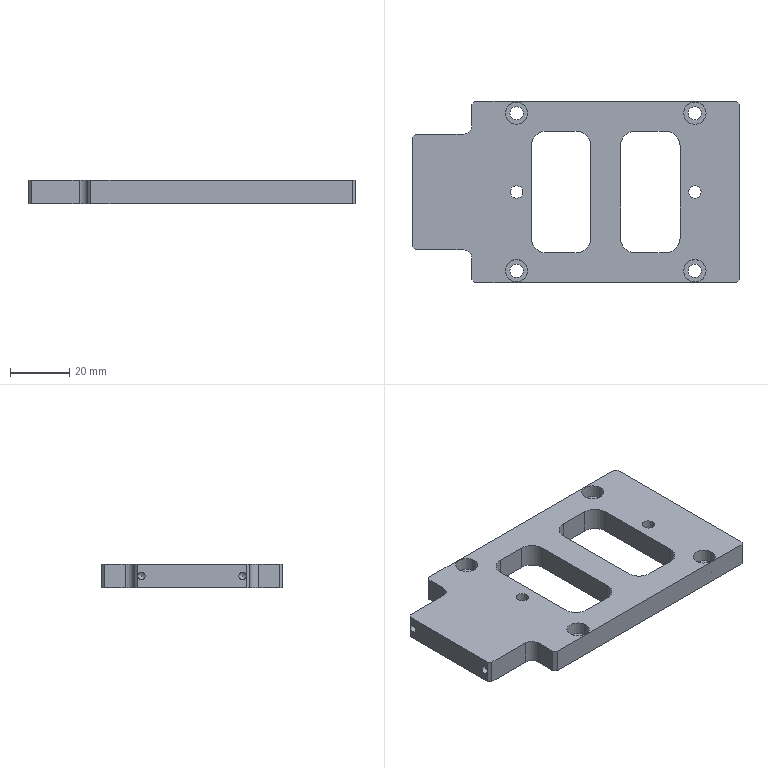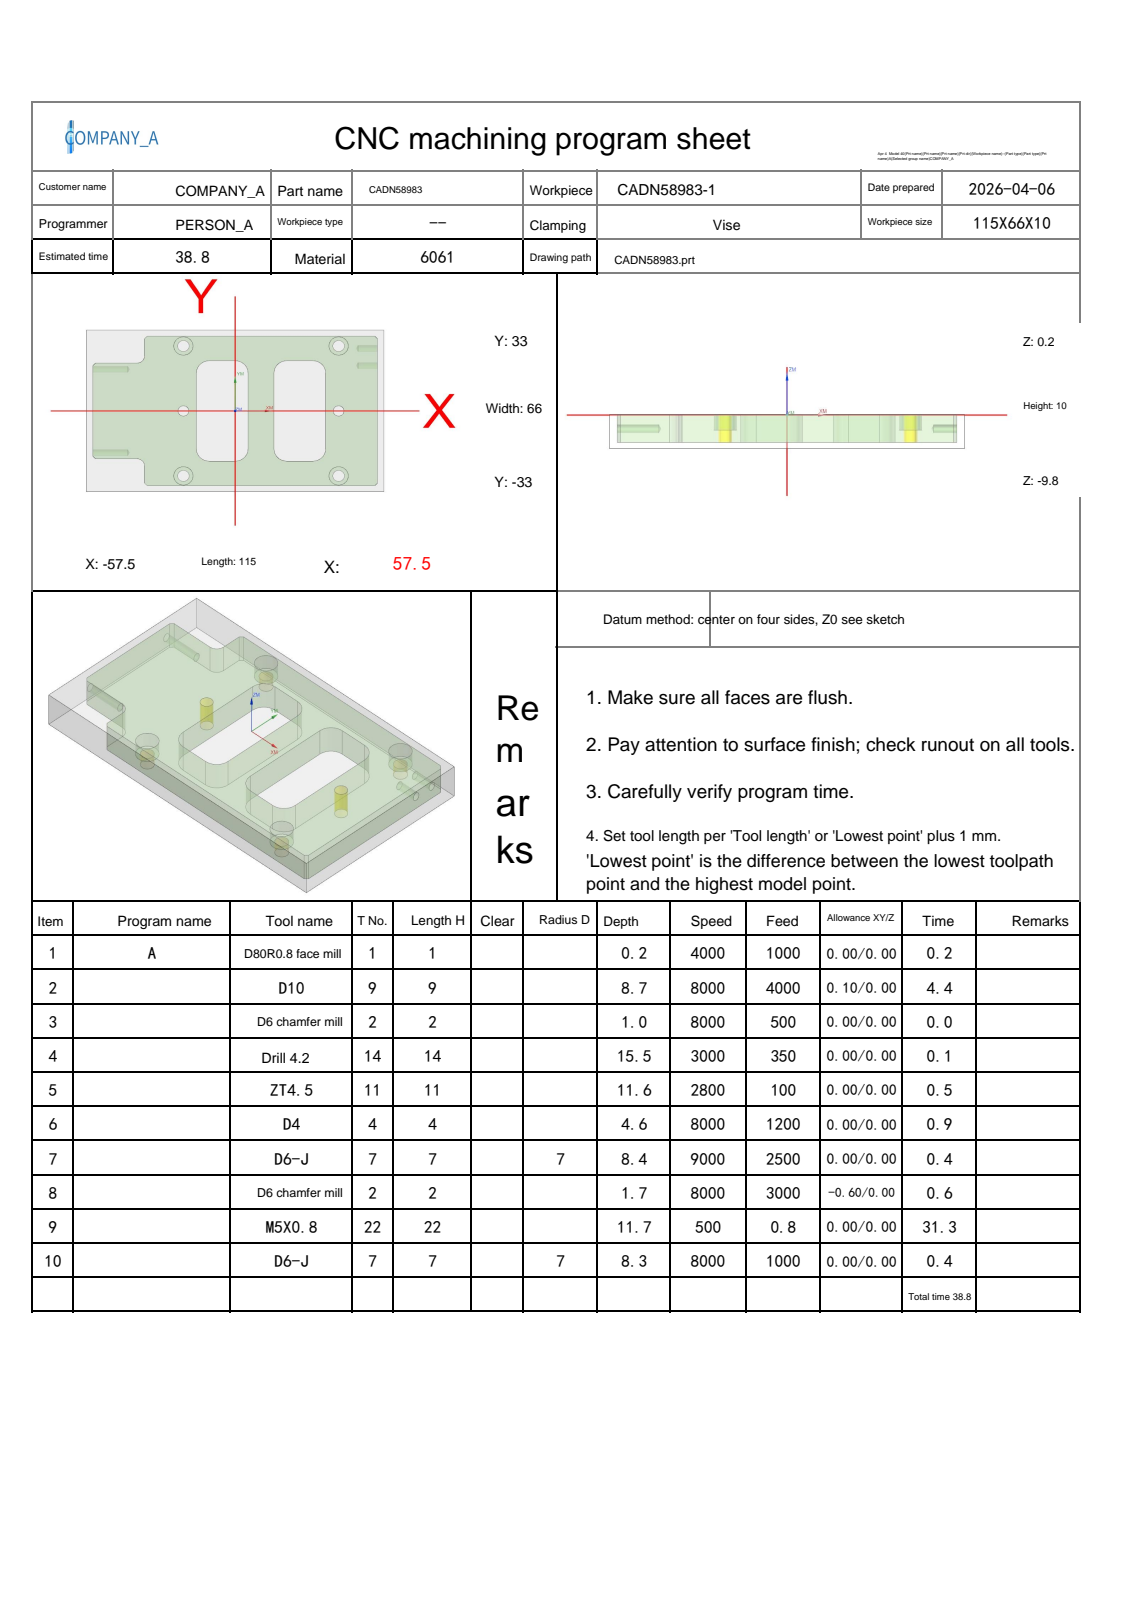NC program | NX | posted by the shop | part box 110 x 61 x 8 mm
Lines 2241 to 4150 of 4510, first 1482 of 1910 lines:
N4 T14 M06
(Drill 4.2 D=4.2 DR_a=118 H=14)
G00 G90 G54 X-20. Y0.0 M03 S3000
G43 H14 Z20.
M08
G98 G83 X-20. Y0.0 Z-15.262 R1. F350. Q3.
X40.
G80
G00 Z20.
G91 G28 Z0.0
M05
M09
G91 G28 Z0.0
M01
N5 T11 M06
(ZT4.5 D=4.5 DR_a=118 H=11)
G00 G90 G54 X40. Y26.5 M03 S2800
G43 H11 Z20.
M08
G98 G83 X40. Y26.5 Z-11.352 R1. F100. Q2.
Y-26.5
X-20.
Y26.5
G80
G00 Z20.
G91 G28 Z0.0
M05
M09
G91 G28 Z0.0
M01
N6 T04 M06
(D4  D=4. R=0. H=04 ce=0.10 di=0.00)
G00 G90 G54 X40. Y26.5 M03 S8000
G43 H04 Z20.
M08
Z.5
G03 X40.825 Y25.675 I.825 J0.0 F1200.
X41.65 Y26.5 I0.0 J.825
X41.65 Y26.5 Z.2 I-1.65 J0.0
X41.65 Y26.5 Z-.1 I-1.65 J0.0
X41.65 Y26.5 Z-.4 I-1.65 J0.0
X41.65 Y26.5 Z-.7 I-1.65 J0.0
X41.65 Y26.5 Z-1. I-1.65 J0.0
X41.65 Y26.5 Z-1.3 I-1.65 J0.0
X41.65 Y26.5 Z-1.6 I-1.65 J0.0
X41.65 Y26.5 Z-1.9 I-1.65 J0.0
X41.65 Y26.5 Z-2.2 I-1.65 J0.0
X41.65 Y26.5 Z-2.5 I-1.65 J0.0
X41.65 Y26.5 Z-2.8 I-1.65 J0.0
X41.65 Y26.5 Z-3.1 I-1.65 J0.0
X41.65 Y26.5 Z-3.4 I-1.65 J0.0
X41.65 Y26.5 Z-3.7 I-1.65 J0.0
X41.65 Y26.5 Z-4. I-1.65 J0.0
X41.65 Y26.5 Z-4.3 I-1.65 J0.0
X39.175 Y27.929 Z-4.4 I-1.65 J0.0
X38.35 Y26.5 I.825 J-1.429
X40. Y24.85 I1.65 J0.0
X41.65 Y26.5 I0.0 J1.65
X40. Y28.15 I-1.65 J0.0
X39.175 Y27.929 I0.0 J-1.65
X38.763 Y27.214 I.413 J-.714
X39.588 Y26.389 I.825 J0.0
X40. Y26.5 I0.0 J.825
G00 Z20.
Y-26.5
Z.5
G03 X40.825 Y-27.325 I.825 J0.0
X41.65 Y-26.5 I0.0 J.825
X41.65 Y-26.5 Z.2 I-1.65 J0.0
X41.65 Y-26.5 Z-.1 I-1.65 J0.0
X41.65 Y-26.5 Z-.4 I-1.65 J0.0
X41.65 Y-26.5 Z-.7 I-1.65 J0.0
X41.65 Y-26.5 Z-1. I-1.65 J0.0
X41.65 Y-26.5 Z-1.3 I-1.65 J0.0
X41.65 Y-26.5 Z-1.6 I-1.65 J0.0
X41.65 Y-26.5 Z-1.9 I-1.65 J0.0
X41.65 Y-26.5 Z-2.2 I-1.65 J0.0
X41.65 Y-26.5 Z-2.5 I-1.65 J0.0
X41.65 Y-26.5 Z-2.8 I-1.65 J0.0
X41.65 Y-26.5 Z-3.1 I-1.65 J0.0
X41.65 Y-26.5 Z-3.4 I-1.65 J0.0
X41.65 Y-26.5 Z-3.7 I-1.65 J0.0
X41.65 Y-26.5 Z-4. I-1.65 J0.0
X41.65 Y-26.5 Z-4.3 I-1.65 J0.0
X39.175 Y-25.071 Z-4.4 I-1.65 J0.0
X38.35 Y-26.5 I.825 J-1.429
X40. Y-28.15 I1.65 J0.0
X41.65 Y-26.5 I0.0 J1.65
X40. Y-24.85 I-1.65 J0.0
X39.175 Y-25.071 I0.0 J-1.65
X38.763 Y-25.786 I.413 J-.714
X39.588 Y-26.611 I.825 J0.0
X40. Y-26.5 I0.0 J.825
G00 Z20.
X-20.
Z.5
G03 X-19.175 Y-27.325 I.825 J0.0
X-18.35 Y-26.5 I0.0 J.825
X-18.35 Y-26.5 Z.2 I-1.65 J0.0
X-18.35 Y-26.5 Z-.1 I-1.65 J0.0
X-18.35 Y-26.5 Z-.4 I-1.65 J0.0
X-18.35 Y-26.5 Z-.7 I-1.65 J0.0
X-18.35 Y-26.5 Z-1. I-1.65 J0.0
X-18.35 Y-26.5 Z-1.3 I-1.65 J0.0
X-18.35 Y-26.5 Z-1.6 I-1.65 J0.0
X-18.35 Y-26.5 Z-1.9 I-1.65 J0.0
X-18.35 Y-26.5 Z-2.2 I-1.65 J0.0
X-18.35 Y-26.5 Z-2.5 I-1.65 J0.0
X-18.35 Y-26.5 Z-2.8 I-1.65 J0.0
X-18.35 Y-26.5 Z-3.1 I-1.65 J0.0
X-18.35 Y-26.5 Z-3.4 I-1.65 J0.0
X-18.35 Y-26.5 Z-3.7 I-1.65 J0.0
X-18.35 Y-26.5 Z-4. I-1.65 J0.0
X-18.35 Y-26.5 Z-4.3 I-1.65 J0.0
X-20.825 Y-25.071 Z-4.4 I-1.65 J0.0
X-21.65 Y-26.5 I.825 J-1.429
X-20. Y-28.15 I1.65 J0.0
X-18.35 Y-26.5 I0.0 J1.65
X-20. Y-24.85 I-1.65 J0.0
X-20.825 Y-25.071 I0.0 J-1.65
X-21.238 Y-25.786 I.413 J-.714
X-20.413 Y-26.611 I.825 J0.0
X-20. Y-26.5 I0.0 J.825
G00 Z20.
Y26.5
Z.5
G03 X-19.175 Y25.675 I.825 J0.0
X-18.35 Y26.5 I0.0 J.825
X-18.35 Y26.5 Z.2 I-1.65 J0.0
X-18.35 Y26.5 Z-.1 I-1.65 J0.0
X-18.35 Y26.5 Z-.4 I-1.65 J0.0
X-18.35 Y26.5 Z-.7 I-1.65 J0.0
X-18.35 Y26.5 Z-1. I-1.65 J0.0
X-18.35 Y26.5 Z-1.3 I-1.65 J0.0
X-18.35 Y26.5 Z-1.6 I-1.65 J0.0
X-18.35 Y26.5 Z-1.9 I-1.65 J0.0
X-18.35 Y26.5 Z-2.2 I-1.65 J0.0
X-18.35 Y26.5 Z-2.5 I-1.65 J0.0
X-18.35 Y26.5 Z-2.8 I-1.65 J0.0
X-18.35 Y26.5 Z-3.1 I-1.65 J0.0
X-18.35 Y26.5 Z-3.4 I-1.65 J0.0
X-18.35 Y26.5 Z-3.7 I-1.65 J0.0
X-18.35 Y26.5 Z-4. I-1.65 J0.0
X-18.35 Y26.5 Z-4.3 I-1.65 J0.0
X-20.825 Y27.929 Z-4.4 I-1.65 J0.0
X-21.65 Y26.5 I.825 J-1.429
X-20. Y24.85 I1.65 J0.0
X-18.35 Y26.5 I0.0 J1.65
X-20. Y28.15 I-1.65 J0.0
X-20.825 Y27.929 I0.0 J-1.65
X-21.238 Y27.214 I.413 J-.714
X-20.413 Y26.389 I.825 J0.0
X-20. Y26.5 I0.0 J.825
G00 Z20.
G00 G90 X40. Y26.5 M03 S8000
Z20.
Z.5
G41 D04
G01 X40.045 Y26.305 F500.
G03 X40.886 Y25.636 I.841 J.195
X41.75 Y26.5 I0.0 J.864
X41.736 Y26.281 Z-4.4 I-1.75 J0.0
X41.75 Y26.5 I-1.736 J.219
X40. Y28.25 I-1.75 J0.0
X38.25 Y26.5 I0.0 J-1.75
X40. Y24.75 I1.75 J0.0
X41.736 Y26.281 I0.0 J1.75
G01 X41.743 Y26.389
G03 X40.879 Y27.252 I-.864 J0.0
X40.069 Y26.688 I0.0 J-.864
G01 G40 X40. Y26.5
G00 Z20.
Y-26.5
Z.5
G41 D04
G01 X40.045 Y-26.695
G03 X40.886 Y-27.364 I.841 J.195
X41.75 Y-26.5 I0.0 J.864
X41.736 Y-26.719 Z-4.4 I-1.75 J0.0
X41.75 Y-26.5 I-1.736 J.219
X40. Y-24.75 I-1.75 J0.0
X38.25 Y-26.5 I0.0 J-1.75
X40. Y-28.25 I1.75 J0.0
X41.736 Y-26.719 I0.0 J1.75
G01 X41.743 Y-26.611
G03 X40.879 Y-25.748 I-.864 J0.0
X40.069 Y-26.312 I0.0 J-.864
G01 G40 X40. Y-26.5
G00 Z20.
X-20.
Z.5
G41 D04
G01 X-19.955 Y-26.695
G03 X-19.114 Y-27.364 I.841 J.195
X-18.25 Y-26.5 I0.0 J.864
X-18.264 Y-26.719 Z-4.4 I-1.75 J0.0
X-18.25 Y-26.5 I-1.736 J.219
X-20. Y-24.75 I-1.75 J0.0
X-21.75 Y-26.5 I0.0 J-1.75
X-20. Y-28.25 I1.75 J0.0
X-18.264 Y-26.719 I0.0 J1.75
G01 X-18.257 Y-26.611
G03 X-19.121 Y-25.748 I-.864 J0.0
X-19.931 Y-26.312 I0.0 J-.864
G01 G40 X-20. Y-26.5
G00 Z20.
Y26.5
Z.5
G41 D04
G01 X-19.955 Y26.305
G03 X-19.114 Y25.636 I.841 J.195
X-18.25 Y26.5 I0.0 J.864
X-18.264 Y26.281 Z-4.4 I-1.75 J0.0
X-18.25 Y26.5 I-1.736 J.219
X-20. Y28.25 I-1.75 J0.0
X-21.75 Y26.5 I0.0 J-1.75
X-20. Y24.75 I1.75 J0.0
X-18.264 Y26.281 I0.0 J1.75
G01 X-18.257 Y26.389
G03 X-19.121 Y27.252 I-.864 J0.0
X-19.931 Y26.688 I0.0 J-.864
G01 G40 X-20. Y26.5
G00 Z20.
G91 G28 Z0.0
M05
M09
G91 G28 Z0.0
M01
N7 T07 M06
(D6-J  D=6. R=0. H=07 ce=0.00 di=0.00)
G00 G90 G54 X29.9 Y-16.5 M03 S6000
G43 H07 Z20.
M08
Z-7.7
G01 Z-8.2 F1000.
G41 D07
X31.
G03 X32. Y-15.5 I0.0 J1.
G01 Y15.5
G03 X30. Y17.5 I-2. J0.0
G01 X20.
G03 X18. Y15.5 I0.0 J-2.
G01 Y-15.5
G03 X20. Y-17.5 I2. J0.0
G01 X30.
G03 X32. Y-15.5 I0.0 J2.
G01 Y-15.
G03 X31. Y-14. I-1. J0.0
G01 G40 X30.9
Z-7.7
G00 Z20.
X-.1 Y-16.5
Z-7.7
G01 Z-8.2
G41 D07
X1.
G03 X2. Y-15.5 I0.0 J1.
G01 Y15.5
G03 X0.0 Y17.5 I-2. J0.0
G01 X-10.
G03 X-12. Y15.5 I0.0 J-2.
G01 Y-15.5
G03 X-10. Y-17.5 I2. J0.0
G01 X0.0
G03 X2. Y-15.5 I0.0 J2.
G01 Y-15.
G03 X1. Y-14. I-1. J0.0
G01 G40 X.9
Z-7.7
G00 Z20.
G00 G90 X-38.919 Y-25.318 M03 S9000
Z20.
Z.606
G01 X-38.909 Y-25.316 Z.477 F2000.
X-38.88 Y-25.312 Z.36
X-38.834 Y-25.303 Z.255
X-38.776 Y-25.291 Z.161
X-38.706 Y-25.275 Z.078
X-38.628 Y-25.254 Z.004
X-38.545 Y-25.228 Z-.06
X-38.46 Y-25.197 Z-.114
X-38.374 Y-25.16 Z-.161
X-38.291 Y-25.118 Z-.2
X-38.213 Y-25.069 Z-.231
X-38.144 Y-25.013 Z-.255
X-38.085 Y-24.95 Z-.273
X-38.039 Y-24.88 Z-.285
X-38.01 Y-24.802 Z-.292
X-38. Y-24.716 Z-.294
Y-22.5 F2500.
X-40.216
X-40.289 Y-22.516 Z-.295
X-40.343 Y-22.563 Z-.298
X-40.381 Y-22.636 Z-.302
X-40.403 Y-22.732 Z-.308
X-40.411 Y-22.845 Z-.314
X-40.406 Y-22.974 Z-.322
X-40.389 Y-23.112 Z-.331
X-40.362 Y-23.258 Z-.341
X-40.325 Y-23.406 Z-.352
X-40.28 Y-23.553 Z-.363
X-40.228 Y-23.694 Z-.374
X-40.117 Y-23.932 Z-.396
X-39.985 Y-24.14 Z-.419
X-39.83 Y-24.321 Z-.442
X-39.649 Y-24.478 Z-.465
X-39.441 Y-24.611 Z-.487
X-39.203 Y-24.723 Z-.509
X-39.061 Y-24.776 Z-.521
X-38.913 Y-24.821 Z-.532
X-38.764 Y-24.859 Z-.542
X-38.618 Y-24.887 Z-.552
X-38.478 Y-24.905 Z-.561
X-38.349 Y-24.91 Z-.569
X-38.234 Y-24.903 Z-.576
X-38.137 Y-24.881 Z-.581
X-38.064 Y-24.843 Z-.585
X-38.017 Y-24.789 Z-.588
X-38. Y-24.716 Z-.589
Y-22.5
X-40.216
X-40.289 Y-22.516 Z-.59
X-40.343 Y-22.563 Z-.592
X-40.381 Y-22.636 Z-.596
X-40.403 Y-22.732 Z-.602
X-40.411 Y-22.845 Z-.609
X-40.406 Y-22.974 Z-.617
X-40.389 Y-23.112 Z-.626
X-40.362 Y-23.258 Z-.635
X-40.325 Y-23.406 Z-.646
X-40.28 Y-23.553 Z-.657
X-40.228 Y-23.694 Z-.669
X-40.117 Y-23.932 Z-.691
X-39.985 Y-24.14 Z-.713
X-39.83 Y-24.321 Z-.736
X-39.649 Y-24.478 Z-.759
X-39.441 Y-24.611 Z-.782
X-39.203 Y-24.723 Z-.804
X-39.061 Y-24.776 Z-.815
X-38.913 Y-24.821 Z-.826
X-38.764 Y-24.859 Z-.837
X-38.618 Y-24.887 Z-.847
X-38.478 Y-24.905 Z-.855
X-38.349 Y-24.91 Z-.863
X-38.234 Y-24.903 Z-.87
X-38.137 Y-24.881 Z-.876
X-38.064 Y-24.843 Z-.88
X-38.017 Y-24.789 Z-.882
X-38. Y-24.716 Z-.883
Y-22.5
X-40.216
X-40.289 Y-22.516 Z-.884
X-40.343 Y-22.563 Z-.887
X-40.381 Y-22.636 Z-.891
X-40.403 Y-22.732 Z-.896
X-40.411 Y-22.845 Z-.903
X-40.406 Y-22.974 Z-.911
X-40.389 Y-23.112 Z-.92
X-40.362 Y-23.258 Z-.93
X-40.325 Y-23.406 Z-.94
X-40.28 Y-23.553 Z-.952
X-40.228 Y-23.694 Z-.963
X-40.117 Y-23.932 Z-.985
X-39.985 Y-24.14 Z-1.008
X-39.83 Y-24.321 Z-1.031
X-39.649 Y-24.478 Z-1.054
X-39.441 Y-24.611 Z-1.076
X-39.203 Y-24.723 Z-1.098
X-39.061 Y-24.776 Z-1.11
X-38.913 Y-24.821 Z-1.121
X-38.764 Y-24.859 Z-1.131
X-38.618 Y-24.887 Z-1.141
X-38.478 Y-24.905 Z-1.15
X-38.349 Y-24.91 Z-1.158
X-38.234 Y-24.903 Z-1.165
X-38.137 Y-24.881 Z-1.17
X-38.064 Y-24.843 Z-1.174
X-38.017 Y-24.789 Z-1.177
X-38. Y-24.716 Z-1.178
Y-22.5
X-40.216
X-40.289 Y-22.516 Z-1.179
X-40.343 Y-22.563 Z-1.181
X-40.381 Y-22.636 Z-1.185
X-40.403 Y-22.732 Z-1.191
X-40.411 Y-22.845 Z-1.198
X-40.406 Y-22.974 Z-1.206
X-40.389 Y-23.112 Z-1.215
X-40.362 Y-23.258 Z-1.224
X-40.325 Y-23.406 Z-1.235
X-40.28 Y-23.553 Z-1.246
X-40.228 Y-23.694 Z-1.258
X-40.117 Y-23.932 Z-1.279
X-39.985 Y-24.14 Z-1.302
X-39.83 Y-24.321 Z-1.325
X-39.649 Y-24.478 Z-1.348
X-39.441 Y-24.611 Z-1.371
X-39.203 Y-24.723 Z-1.392
X-39.061 Y-24.776 Z-1.404
X-38.913 Y-24.821 Z-1.415
X-38.764 Y-24.859 Z-1.426
X-38.618 Y-24.887 Z-1.435
X-38.478 Y-24.905 Z-1.444
X-38.349 Y-24.91 Z-1.452
X-38.234 Y-24.903 Z-1.459
X-38.137 Y-24.881 Z-1.465
X-38.064 Y-24.843 Z-1.469
X-38.017 Y-24.789 Z-1.471
X-38. Y-24.716 Z-1.472
Y-22.5
X-40.216
X-40.289 Y-22.516 Z-1.473
X-40.343 Y-22.563 Z-1.476
X-40.381 Y-22.636 Z-1.48
X-40.403 Y-22.732 Z-1.485
X-40.411 Y-22.845 Z-1.492
X-40.406 Y-22.974 Z-1.5
X-40.389 Y-23.112 Z-1.509
X-40.362 Y-23.258 Z-1.519
X-40.325 Y-23.406 Z-1.529
X-40.28 Y-23.553 Z-1.54
X-40.228 Y-23.694 Z-1.552
X-40.117 Y-23.932 Z-1.574
X-39.985 Y-24.14 Z-1.596
X-39.83 Y-24.321 Z-1.619
X-39.649 Y-24.478 Z-1.642
X-39.441 Y-24.611 Z-1.665
X-39.203 Y-24.723 Z-1.687
X-39.061 Y-24.776 Z-1.698
X-38.913 Y-24.821 Z-1.71
X-38.764 Y-24.859 Z-1.72
X-38.618 Y-24.887 Z-1.73
X-38.478 Y-24.905 Z-1.739
X-38.349 Y-24.91 Z-1.747
X-38.234 Y-24.903 Z-1.754
X-38.137 Y-24.881 Z-1.759
X-38.064 Y-24.843 Z-1.763
X-38.017 Y-24.789 Z-1.766
X-38. Y-24.716 Z-1.767
Y-22.5
X-40.216
X-40.289 Y-22.516 Z-1.768
X-40.343 Y-22.563 Z-1.77
X-40.381 Y-22.636 Z-1.774
X-40.403 Y-22.732 Z-1.78
X-40.411 Y-22.845 Z-1.787
X-40.406 Y-22.974 Z-1.795
X-40.389 Y-23.112 Z-1.803
X-40.362 Y-23.258 Z-1.813
X-40.325 Y-23.406 Z-1.824
X-40.28 Y-23.553 Z-1.835
X-40.228 Y-23.694 Z-1.846
X-40.117 Y-23.932 Z-1.868
X-39.985 Y-24.14 Z-1.891
X-39.83 Y-24.321 Z-1.914
X-39.649 Y-24.478 Z-1.937
X-39.441 Y-24.611 Z-1.959
X-39.203 Y-24.723 Z-1.981
X-39.061 Y-24.776 Z-1.993
X-38.913 Y-24.821 Z-2.004
X-38.764 Y-24.859 Z-2.015
X-38.618 Y-24.887 Z-2.024
X-38.478 Y-24.905 Z-2.033
X-38.349 Y-24.91 Z-2.041
X-38.234 Y-24.903 Z-2.048
X-38.137 Y-24.881 Z-2.054
X-38.064 Y-24.843 Z-2.058
X-38.017 Y-24.789 Z-2.06
X-38. Y-24.716 Z-2.061
Y-22.5
X-40.216
X-40.289 Y-22.516 Z-2.062
X-40.343 Y-22.563 Z-2.065
X-40.381 Y-22.636 Z-2.069
X-40.403 Y-22.732 Z-2.074
X-40.411 Y-22.845 Z-2.081
X-40.406 Y-22.974 Z-2.089
X-40.389 Y-23.112 Z-2.098
X-40.362 Y-23.258 Z-2.108
X-40.325 Y-23.406 Z-2.118
X-40.28 Y-23.553 Z-2.129
X-40.228 Y-23.694 Z-2.141
X-40.117 Y-23.932 Z-2.163
X-39.985 Y-24.14 Z-2.185
X-39.83 Y-24.321 Z-2.208
X-39.649 Y-24.478 Z-2.231
X-39.441 Y-24.611 Z-2.254
X-39.203 Y-24.723 Z-2.276
X-39.061 Y-24.776 Z-2.287
X-38.913 Y-24.821 Z-2.298
X-38.764 Y-24.859 Z-2.309
X-38.618 Y-24.887 Z-2.319
X-38.478 Y-24.905 Z-2.328
X-38.349 Y-24.91 Z-2.336
X-38.234 Y-24.903 Z-2.342
X-38.137 Y-24.881 Z-2.348
X-38.064 Y-24.843 Z-2.352
X-38.017 Y-24.789 Z-2.355
X-38. Y-24.716 Z-2.356
Y-22.5
X-40.216
X-40.289 Y-22.516
X-40.343 Y-22.563 Z-2.359
X-40.381 Y-22.636 Z-2.363
X-40.403 Y-22.732 Z-2.369
X-40.411 Y-22.845 Z-2.375
X-40.406 Y-22.974 Z-2.383
X-40.389 Y-23.112 Z-2.392
X-40.362 Y-23.258 Z-2.402
X-40.325 Y-23.406 Z-2.413
X-40.28 Y-23.553 Z-2.424
X-40.228 Y-23.694 Z-2.435
X-40.117 Y-23.932 Z-2.457
X-39.985 Y-24.14 Z-2.48
X-39.83 Y-24.321 Z-2.503
X-39.649 Y-24.478 Z-2.526
X-39.441 Y-24.611 Z-2.548
X-39.203 Y-24.723 Z-2.57
X-39.061 Y-24.776 Z-2.582
X-38.913 Y-24.821 Z-2.593
X-38.764 Y-24.859 Z-2.603
X-38.618 Y-24.887 Z-2.613
X-38.478 Y-24.905 Z-2.622
X-38.349 Y-24.91 Z-2.63
X-38.234 Y-24.903 Z-2.637
X-38.137 Y-24.881 Z-2.642
X-38.064 Y-24.843 Z-2.647
X-38.017 Y-24.789 Z-2.649
X-38. Y-24.716 Z-2.65
Y-22.5
X-40.216
X-40.289 Y-22.516 Z-2.651
X-40.343 Y-22.563 Z-2.653
X-40.381 Y-22.636 Z-2.658
X-40.403 Y-22.732 Z-2.663
X-40.411 Y-22.845 Z-2.67
X-40.406 Y-22.974 Z-2.678
X-40.389 Y-23.112 Z-2.687
X-40.362 Y-23.258 Z-2.697
X-40.325 Y-23.406 Z-2.707
X-40.28 Y-23.553 Z-2.718
X-40.228 Y-23.694 Z-2.73
X-40.117 Y-23.932 Z-2.752
X-39.985 Y-24.14 Z-2.774
X-39.83 Y-24.321 Z-2.797
X-39.649 Y-24.478 Z-2.82
X-39.441 Y-24.611 Z-2.843
X-39.203 Y-24.723 Z-2.865
X-39.061 Y-24.776 Z-2.876
X-38.913 Y-24.821 Z-2.887
X-38.764 Y-24.859 Z-2.898
X-38.618 Y-24.887 Z-2.908
X-38.478 Y-24.905 Z-2.917
X-38.349 Y-24.91 Z-2.925
X-38.234 Y-24.903 Z-2.931
X-38.137 Y-24.881 Z-2.937
X-38.064 Y-24.843 Z-2.941
X-38.017 Y-24.789 Z-2.944
X-38. Y-24.716
Y-22.5
X-40.216
X-40.289 Y-22.516 Z-2.945
X-40.343 Y-22.563 Z-2.948
X-40.381 Y-22.636 Z-2.952
X-40.403 Y-22.732 Z-2.958
X-40.411 Y-22.845 Z-2.964
X-40.406 Y-22.974 Z-2.972
X-40.389 Y-23.112 Z-2.981
X-40.362 Y-23.258 Z-2.991
X-40.325 Y-23.406 Z-3.002
X-40.28 Y-23.553 Z-3.013
X-40.228 Y-23.694 Z-3.024
X-40.117 Y-23.932 Z-3.046
X-39.985 Y-24.14 Z-3.069
X-39.83 Y-24.321 Z-3.092
X-39.649 Y-24.478 Z-3.115
X-39.441 Y-24.611 Z-3.137
X-39.203 Y-24.723 Z-3.159
X-39.061 Y-24.776 Z-3.171
X-38.913 Y-24.821 Z-3.182
X-38.764 Y-24.859 Z-3.192
X-38.618 Y-24.887 Z-3.202
X-38.478 Y-24.905 Z-3.211
X-38.349 Y-24.91 Z-3.219
X-38.234 Y-24.903 Z-3.226
X-38.137 Y-24.881 Z-3.231
X-38.064 Y-24.843 Z-3.235
X-38.017 Y-24.789 Z-3.238
X-38. Y-24.716 Z-3.239
Y-22.5
X-40.216
X-40.289 Y-22.516 Z-3.24
X-40.343 Y-22.563 Z-3.242
X-40.381 Y-22.636 Z-3.246
X-40.403 Y-22.732 Z-3.252
X-40.411 Y-22.845 Z-3.259
X-40.406 Y-22.974 Z-3.267
X-40.389 Y-23.112 Z-3.276
X-40.362 Y-23.258 Z-3.285
X-40.325 Y-23.406 Z-3.296
X-40.28 Y-23.553 Z-3.307
X-40.228 Y-23.694 Z-3.319
X-40.117 Y-23.932 Z-3.341
X-39.985 Y-24.14 Z-3.363
X-39.83 Y-24.321 Z-3.386
X-39.649 Y-24.478 Z-3.409
X-39.441 Y-24.611 Z-3.432
X-39.203 Y-24.723 Z-3.454
X-39.061 Y-24.776 Z-3.465
X-38.913 Y-24.821 Z-3.476
X-38.764 Y-24.859 Z-3.487
X-38.618 Y-24.887 Z-3.497
X-38.478 Y-24.905 Z-3.505
X-38.349 Y-24.91 Z-3.513
X-38.234 Y-24.903 Z-3.52
X-38.137 Y-24.881 Z-3.526
X-38.064 Y-24.843 Z-3.53
X-38.017 Y-24.789 Z-3.532
X-38. Y-24.716 Z-3.533
Y-22.5
X-40.216
X-40.289 Y-22.516 Z-3.534
X-40.343 Y-22.563 Z-3.537
X-40.381 Y-22.636 Z-3.541
X-40.403 Y-22.732 Z-3.546
X-40.411 Y-22.845 Z-3.553
X-40.406 Y-22.974 Z-3.561
X-40.389 Y-23.112 Z-3.57
X-40.362 Y-23.258 Z-3.58
X-40.325 Y-23.406 Z-3.59
X-40.28 Y-23.553 Z-3.602
X-40.228 Y-23.694 Z-3.613
X-40.117 Y-23.932 Z-3.635
X-39.985 Y-24.14 Z-3.658
X-39.83 Y-24.321 Z-3.681
X-39.649 Y-24.478 Z-3.704
X-39.441 Y-24.611 Z-3.726
X-39.203 Y-24.723 Z-3.748
X-39.061 Y-24.776 Z-3.76
X-38.913 Y-24.821 Z-3.771
X-38.764 Y-24.859 Z-3.781
X-38.618 Y-24.887 Z-3.791
X-38.478 Y-24.905 Z-3.8
X-38.349 Y-24.91 Z-3.808
X-38.234 Y-24.903 Z-3.815
X-38.137 Y-24.881 Z-3.82
X-38.064 Y-24.843 Z-3.824
X-38.017 Y-24.789 Z-3.827
X-38. Y-24.716 Z-3.828
Y-22.5
X-40.216
X-40.289 Y-22.516 Z-3.829
X-40.343 Y-22.563 Z-3.831
X-40.381 Y-22.636 Z-3.835
X-40.403 Y-22.732 Z-3.841
X-40.411 Y-22.845 Z-3.848
X-40.406 Y-22.974 Z-3.856
X-40.389 Y-23.112 Z-3.865
X-40.362 Y-23.258 Z-3.874
X-40.325 Y-23.406 Z-3.885
X-40.28 Y-23.553 Z-3.896
X-40.228 Y-23.694 Z-3.908
X-40.117 Y-23.932 Z-3.929
X-39.985 Y-24.14 Z-3.952
X-39.83 Y-24.321 Z-3.975
X-39.649 Y-24.478 Z-3.998
X-39.441 Y-24.611 Z-4.021
X-39.203 Y-24.723 Z-4.042
X-39.061 Y-24.776 Z-4.054
X-38.913 Y-24.821 Z-4.065
X-38.764 Y-24.859 Z-4.076
X-38.618 Y-24.887 Z-4.085
X-38.478 Y-24.905 Z-4.094
X-38.349 Y-24.91 Z-4.102
X-38.234 Y-24.903 Z-4.109
X-38.137 Y-24.881 Z-4.115
X-38.064 Y-24.843 Z-4.119
X-38.017 Y-24.789 Z-4.121
X-38. Y-24.716 Z-4.122
Y-22.5
X-40.216
X-40.289 Y-22.516 Z-4.123
X-40.343 Y-22.563 Z-4.126
X-40.381 Y-22.636 Z-4.13
X-40.403 Y-22.732 Z-4.135
X-40.411 Y-22.845 Z-4.142
X-40.406 Y-22.974 Z-4.15
X-40.389 Y-23.112 Z-4.159
X-40.362 Y-23.258 Z-4.169
X-40.325 Y-23.406 Z-4.179
X-40.28 Y-23.553 Z-4.19
X-40.228 Y-23.694 Z-4.202
X-40.117 Y-23.932 Z-4.224
X-39.985 Y-24.14 Z-4.246
X-39.83 Y-24.321 Z-4.269
X-39.649 Y-24.478 Z-4.292
X-39.441 Y-24.611 Z-4.315
X-39.203 Y-24.723 Z-4.337
X-39.061 Y-24.776 Z-4.348
X-38.913 Y-24.821 Z-4.36
X-38.764 Y-24.859 Z-4.37
X-38.618 Y-24.887 Z-4.38
X-38.478 Y-24.905 Z-4.389
X-38.349 Y-24.91 Z-4.397
X-38.234 Y-24.903 Z-4.404
X-38.137 Y-24.881 Z-4.409
X-38.064 Y-24.843 Z-4.413
X-38.017 Y-24.789 Z-4.416
X-38. Y-24.716 Z-4.417
Y-22.5
X-40.216
X-40.289 Y-22.516 Z-4.418
X-40.343 Y-22.563 Z-4.42
X-40.381 Y-22.636 Z-4.424
X-40.403 Y-22.732 Z-4.43
X-40.411 Y-22.845 Z-4.437
X-40.406 Y-22.974 Z-4.445
X-40.389 Y-23.112 Z-4.453
X-40.362 Y-23.258 Z-4.463
X-40.325 Y-23.406 Z-4.474
X-40.28 Y-23.553 Z-4.485
X-40.228 Y-23.694 Z-4.496
X-40.117 Y-23.932 Z-4.518
X-39.985 Y-24.14 Z-4.541
X-39.83 Y-24.321 Z-4.564
X-39.649 Y-24.478 Z-4.587
X-39.441 Y-24.611 Z-4.609
X-39.203 Y-24.723 Z-4.631
X-39.061 Y-24.776 Z-4.643
X-38.913 Y-24.821 Z-4.654
X-38.764 Y-24.859 Z-4.665
X-38.618 Y-24.887 Z-4.674
X-38.478 Y-24.905 Z-4.683
X-38.349 Y-24.91 Z-4.691
X-38.234 Y-24.903 Z-4.698
X-38.137 Y-24.881 Z-4.704
X-38.064 Y-24.843 Z-4.708
X-38.017 Y-24.789 Z-4.71
X-38. Y-24.716 Z-4.711
Y-22.5
X-40.216
X-40.289 Y-22.516 Z-4.712
X-40.343 Y-22.563 Z-4.715
X-40.381 Y-22.636 Z-4.719
X-40.403 Y-22.732 Z-4.724
X-40.411 Y-22.845 Z-4.731
X-40.406 Y-22.974 Z-4.739
X-40.389 Y-23.112 Z-4.748
X-40.362 Y-23.258 Z-4.758
X-40.325 Y-23.406 Z-4.768
X-40.28 Y-23.553 Z-4.779
X-40.228 Y-23.694 Z-4.791
X-40.117 Y-23.932 Z-4.813
X-39.985 Y-24.14 Z-4.835
X-39.83 Y-24.321 Z-4.858
X-39.649 Y-24.478 Z-4.881
X-39.441 Y-24.611 Z-4.904
X-39.203 Y-24.723 Z-4.926
X-39.061 Y-24.776 Z-4.937
X-38.913 Y-24.821 Z-4.948
X-38.764 Y-24.859 Z-4.959
X-38.618 Y-24.887 Z-4.969
X-38.478 Y-24.905 Z-4.978
X-38.349 Y-24.91 Z-4.986
X-38.234 Y-24.903 Z-4.992
X-38.137 Y-24.881 Z-4.998
X-38.064 Y-24.843 Z-5.002
X-38.017 Y-24.789 Z-5.005
X-38. Y-24.716 Z-5.006
Y-22.5
X-40.216
X-40.289 Y-22.516
X-40.343 Y-22.563 Z-5.009
X-40.381 Y-22.636 Z-5.013
X-40.403 Y-22.732 Z-5.019
X-40.411 Y-22.845 Z-5.025
X-40.406 Y-22.974 Z-5.033
X-40.389 Y-23.112 Z-5.042
X-40.362 Y-23.258 Z-5.052
X-40.325 Y-23.406 Z-5.063
X-40.28 Y-23.553 Z-5.074
X-40.228 Y-23.694 Z-5.085
X-40.117 Y-23.932 Z-5.107
X-39.985 Y-24.14 Z-5.13
X-39.83 Y-24.321 Z-5.153
X-39.649 Y-24.478 Z-5.176
X-39.441 Y-24.611 Z-5.198
X-39.203 Y-24.723 Z-5.22
X-39.061 Y-24.776 Z-5.232
X-38.913 Y-24.821 Z-5.243
X-38.764 Y-24.859 Z-5.253
X-38.618 Y-24.887 Z-5.263
X-38.478 Y-24.905 Z-5.272
X-38.349 Y-24.91 Z-5.28
X-38.234 Y-24.903 Z-5.287
X-38.137 Y-24.881 Z-5.292
X-38.064 Y-24.843 Z-5.297
X-38.017 Y-24.789 Z-5.299
X-38. Y-24.716 Z-5.3
Y-22.5
X-40.216
X-40.289 Y-22.516 Z-5.301
X-40.343 Y-22.563 Z-5.303
X-40.381 Y-22.636 Z-5.308
X-40.403 Y-22.732 Z-5.313
X-40.411 Y-22.845 Z-5.32
X-40.406 Y-22.974 Z-5.328
X-40.389 Y-23.112 Z-5.337
X-40.362 Y-23.258 Z-5.347
X-40.325 Y-23.406 Z-5.357
X-40.28 Y-23.553 Z-5.368
X-40.228 Y-23.694 Z-5.38
X-40.117 Y-23.932 Z-5.402
X-39.985 Y-24.14 Z-5.424
X-39.83 Y-24.321 Z-5.447
X-39.649 Y-24.478 Z-5.47
X-39.441 Y-24.611 Z-5.493
X-39.203 Y-24.723 Z-5.515
X-39.061 Y-24.776 Z-5.526
X-38.913 Y-24.821 Z-5.537
X-38.764 Y-24.859 Z-5.548
X-38.618 Y-24.887 Z-5.558
X-38.478 Y-24.905 Z-5.567
X-38.349 Y-24.91 Z-5.575
X-38.234 Y-24.903 Z-5.581
X-38.137 Y-24.881 Z-5.587
X-38.064 Y-24.843 Z-5.591
X-38.017 Y-24.789 Z-5.594
X-38. Y-24.716
Y-22.5
X-40.216
X-40.289 Y-22.516 Z-5.595
X-40.343 Y-22.563 Z-5.598
X-40.381 Y-22.636 Z-5.602
X-40.403 Y-22.732 Z-5.608
X-40.411 Y-22.845 Z-5.614
X-40.406 Y-22.974 Z-5.622
X-40.389 Y-23.112 Z-5.631
X-40.362 Y-23.258 Z-5.641
X-40.325 Y-23.406 Z-5.652
X-40.28 Y-23.553 Z-5.663
X-40.228 Y-23.694 Z-5.674
X-40.117 Y-23.932 Z-5.696
X-39.985 Y-24.14 Z-5.719
X-39.83 Y-24.321 Z-5.742
X-39.649 Y-24.478 Z-5.765
X-39.441 Y-24.611 Z-5.787
X-39.203 Y-24.723 Z-5.809
X-39.061 Y-24.776 Z-5.821
X-38.913 Y-24.821 Z-5.832
X-38.764 Y-24.859 Z-5.842
X-38.618 Y-24.887 Z-5.852
X-38.478 Y-24.905 Z-5.861
X-38.349 Y-24.91 Z-5.869
X-38.234 Y-24.903 Z-5.876
X-38.137 Y-24.881 Z-5.881
X-38.064 Y-24.843 Z-5.885
X-38.017 Y-24.789 Z-5.888
X-38. Y-24.716 Z-5.889
Y-22.5
X-40.216
X-40.289 Y-22.516 Z-5.89
X-40.343 Y-22.563 Z-5.892
X-40.381 Y-22.636 Z-5.896
X-40.403 Y-22.732 Z-5.902
X-40.411 Y-22.845 Z-5.909
X-40.406 Y-22.974 Z-5.917
X-40.389 Y-23.112 Z-5.926
X-40.362 Y-23.258 Z-5.935
X-40.325 Y-23.406 Z-5.946
X-40.28 Y-23.553 Z-5.957
X-40.228 Y-23.694 Z-5.969
X-40.117 Y-23.932 Z-5.991
X-39.985 Y-24.14 Z-6.013
X-39.83 Y-24.321 Z-6.036
X-39.649 Y-24.478 Z-6.059
X-39.441 Y-24.611 Z-6.082
X-39.203 Y-24.723 Z-6.104
X-39.061 Y-24.776 Z-6.115
X-38.913 Y-24.821 Z-6.126
X-38.764 Y-24.859 Z-6.137
X-38.618 Y-24.887 Z-6.147
X-38.478 Y-24.905 Z-6.155
X-38.349 Y-24.91 Z-6.163
X-38.234 Y-24.903 Z-6.17
X-38.137 Y-24.881 Z-6.176
X-38.064 Y-24.843 Z-6.18
X-38.017 Y-24.789 Z-6.182
X-38. Y-24.716 Z-6.183
Y-22.5
X-40.216
X-40.289 Y-22.516 Z-6.184
X-40.343 Y-22.563 Z-6.187
X-40.381 Y-22.636 Z-6.191
X-40.403 Y-22.732 Z-6.196
X-40.411 Y-22.845 Z-6.203
X-40.406 Y-22.974 Z-6.211
X-40.389 Y-23.112 Z-6.22
X-40.362 Y-23.258 Z-6.23
X-40.325 Y-23.406 Z-6.24
X-40.28 Y-23.553 Z-6.252
X-40.228 Y-23.694 Z-6.263
X-40.117 Y-23.932 Z-6.285
X-39.985 Y-24.14 Z-6.308
X-39.83 Y-24.321 Z-6.331
X-39.649 Y-24.478 Z-6.354
X-39.441 Y-24.611 Z-6.376
X-39.203 Y-24.723 Z-6.398
X-39.061 Y-24.776 Z-6.41
X-38.913 Y-24.821 Z-6.421
X-38.764 Y-24.859 Z-6.431
X-38.618 Y-24.887 Z-6.441
X-38.478 Y-24.905 Z-6.45
X-38.349 Y-24.91 Z-6.458
X-38.234 Y-24.903 Z-6.465
X-38.137 Y-24.881 Z-6.47
X-38.064 Y-24.843 Z-6.474
X-38.017 Y-24.789 Z-6.477
X-38. Y-24.716 Z-6.478
Y-22.5
X-40.216
X-40.289 Y-22.516 Z-6.479
X-40.343 Y-22.563 Z-6.481
X-40.381 Y-22.636 Z-6.485
X-40.403 Y-22.732 Z-6.491
X-40.411 Y-22.845 Z-6.498
X-40.406 Y-22.974 Z-6.506
X-40.389 Y-23.112 Z-6.515
X-40.362 Y-23.258 Z-6.524
X-40.325 Y-23.406 Z-6.535
X-40.28 Y-23.553 Z-6.546
X-40.228 Y-23.694 Z-6.558
X-40.117 Y-23.932 Z-6.579
X-39.985 Y-24.14 Z-6.602
X-39.83 Y-24.321 Z-6.625
X-39.649 Y-24.478 Z-6.648
X-39.441 Y-24.611 Z-6.671
X-39.203 Y-24.723 Z-6.692
X-39.061 Y-24.776 Z-6.704
X-38.913 Y-24.821 Z-6.715
X-38.764 Y-24.859 Z-6.726
X-38.618 Y-24.887 Z-6.735
X-38.478 Y-24.905 Z-6.744
X-38.349 Y-24.91 Z-6.752
X-38.234 Y-24.903 Z-6.759
X-38.137 Y-24.881 Z-6.765
X-38.064 Y-24.843 Z-6.769
X-38.017 Y-24.789 Z-6.771
X-38. Y-24.716 Z-6.772
Y-22.5
X-40.216
X-40.289 Y-22.516 Z-6.773
X-40.343 Y-22.563 Z-6.776
X-40.381 Y-22.636 Z-6.78
X-40.403 Y-22.732 Z-6.785
X-40.411 Y-22.845 Z-6.792
X-40.406 Y-22.974 Z-6.8
X-40.389 Y-23.112 Z-6.809
X-40.362 Y-23.258 Z-6.819
X-40.325 Y-23.406 Z-6.829
X-40.28 Y-23.553 Z-6.84
X-40.228 Y-23.694 Z-6.852
X-40.117 Y-23.932 Z-6.874
X-39.985 Y-24.14 Z-6.896
X-39.83 Y-24.321 Z-6.919
X-39.649 Y-24.478 Z-6.942
X-39.441 Y-24.611 Z-6.965
X-39.203 Y-24.723 Z-6.987
X-39.061 Y-24.776 Z-6.998
X-38.913 Y-24.821 Z-7.01
X-38.764 Y-24.859 Z-7.02
X-38.618 Y-24.887 Z-7.03
X-38.478 Y-24.905 Z-7.039
X-38.349 Y-24.91 Z-7.047
X-38.234 Y-24.903 Z-7.054
X-38.137 Y-24.881 Z-7.059
X-38.064 Y-24.843 Z-7.063
X-38.017 Y-24.789 Z-7.066
X-38. Y-24.716 Z-7.067
Y-22.5
X-40.216
X-40.289 Y-22.516 Z-7.068
X-40.343 Y-22.563 Z-7.07
X-40.381 Y-22.636 Z-7.074
X-40.403 Y-22.732 Z-7.08
X-40.411 Y-22.845 Z-7.087
X-40.406 Y-22.974 Z-7.095
X-40.389 Y-23.112 Z-7.103
X-40.362 Y-23.258 Z-7.113
X-40.325 Y-23.406 Z-7.124
X-40.28 Y-23.553 Z-7.135
X-40.228 Y-23.694 Z-7.146
X-40.117 Y-23.932 Z-7.168
X-39.985 Y-24.14 Z-7.191
X-39.83 Y-24.321 Z-7.214
X-39.649 Y-24.478 Z-7.237
X-39.441 Y-24.611 Z-7.259
X-39.203 Y-24.723 Z-7.281
X-39.061 Y-24.776 Z-7.293
X-38.913 Y-24.821 Z-7.304
X-38.764 Y-24.859 Z-7.315
X-38.618 Y-24.887 Z-7.324
X-38.478 Y-24.905 Z-7.333
X-38.349 Y-24.91 Z-7.341
X-38.234 Y-24.903 Z-7.348
X-38.137 Y-24.881 Z-7.354
X-38.064 Y-24.843 Z-7.358
X-38.017 Y-24.789 Z-7.36
X-38. Y-24.716 Z-7.361
Y-22.5
X-40.216
X-40.289 Y-22.516 Z-7.362
X-40.343 Y-22.563 Z-7.365
X-40.381 Y-22.636 Z-7.369
X-40.403 Y-22.732 Z-7.374
X-40.411 Y-22.845 Z-7.381
X-40.406 Y-22.974 Z-7.389
X-40.389 Y-23.112 Z-7.398
X-40.362 Y-23.258 Z-7.408
X-40.325 Y-23.406 Z-7.418
X-40.28 Y-23.553 Z-7.429
X-40.228 Y-23.694 Z-7.441
X-40.117 Y-23.932 Z-7.463
X-39.985 Y-24.14 Z-7.485
X-39.83 Y-24.321 Z-7.508
X-39.649 Y-24.478 Z-7.531
X-39.441 Y-24.611 Z-7.554
X-39.203 Y-24.723 Z-7.576
X-39.061 Y-24.776 Z-7.587
X-38.913 Y-24.821 Z-7.598
X-38.764 Y-24.859 Z-7.609
X-38.618 Y-24.887 Z-7.619
X-38.478 Y-24.905 Z-7.628
X-38.349 Y-24.91 Z-7.636
X-38.234 Y-24.903 Z-7.642
X-38.137 Y-24.881 Z-7.648
X-38.064 Y-24.843 Z-7.652
X-38.017 Y-24.789 Z-7.655
X-38. Y-24.716 Z-7.656
Y-22.5
X-40.216
X-40.289 Y-22.516
X-40.343 Y-22.563 Z-7.659
X-40.381 Y-22.636 Z-7.663
X-40.403 Y-22.732 Z-7.669
X-40.411 Y-22.845 Z-7.675
X-40.406 Y-22.974 Z-7.683
X-40.389 Y-23.112 Z-7.692
X-40.362 Y-23.258 Z-7.702
X-40.325 Y-23.406 Z-7.713
X-40.28 Y-23.553 Z-7.724
X-40.228 Y-23.694 Z-7.735
X-40.117 Y-23.932 Z-7.757
X-39.985 Y-24.14 Z-7.78
X-39.83 Y-24.321 Z-7.803
X-39.649 Y-24.478 Z-7.826
X-39.441 Y-24.611 Z-7.848
X-39.203 Y-24.723 Z-7.87
X-39.061 Y-24.776 Z-7.882
X-38.913 Y-24.821 Z-7.893
X-38.764 Y-24.859 Z-7.903
X-38.618 Y-24.887 Z-7.913
X-38.478 Y-24.905 Z-7.922
X-38.349 Y-24.91 Z-7.93
X-38.234 Y-24.903 Z-7.937
X-38.137 Y-24.881 Z-7.942
X-38.064 Y-24.843 Z-7.947
X-38.017 Y-24.789 Z-7.949
X-38. Y-24.716 Z-7.95
Y-22.5
X-40.216
X-40.302 Y-22.51 Z-7.948
X-40.38 Y-22.539 Z-7.941
X-40.45 Y-22.583 Z-7.929
X-40.513 Y-22.641 Z-7.911
X-40.568 Y-22.709 Z-7.886
X-40.617 Y-22.785 Z-7.855
X-40.66 Y-22.866 Z-7.816
X-40.696 Y-22.95 Z-7.77
X-40.727 Y-23.034 Z-7.715
X-40.753 Y-23.115 Z-7.651
X-40.774 Y-23.191 Z-7.578
X-40.79 Y-23.259 Z-7.494
X-40.802 Y-23.317 Z-7.4
X-40.81 Y-23.361 Z-7.295
X-40.815 Y-23.39 Z-7.179
X-40.816 Y-23.4 Z-7.05
G00 Z20.
Y23.4
Z.606
G01 X-40.815 Y23.39 Z.477 F2000.
X-40.81 Y23.361 Z.36
X-40.802 Y23.317 Z.255
X-40.79 Y23.259 Z.161
X-40.774 Y23.191 Z.078
X-40.753 Y23.115 Z.004
X-40.727 Y23.034 Z-.06
X-40.696 Y22.95 Z-.114
X-40.66 Y22.866 Z-.161
X-40.617 Y22.785 Z-.2
X-40.568 Y22.709 Z-.231
X-40.513 Y22.641 Z-.255
X-40.45 Y22.583 Z-.273
X-40.38 Y22.539 Z-.285
X-40.302 Y22.51 Z-.292
X-40.216 Y22.5 Z-.294
X-38. F2500.
Y24.716
X-38.016 Y24.789 Z-.295
X-38.063 Y24.843 Z-.298
X-38.136 Y24.881 Z-.302
X-38.231 Y24.902 Z-.308
X-38.345 Y24.91 Z-.314
X-38.474 Y24.904 Z-.322
X-38.612 Y24.887 Z-.331
X-38.758 Y24.859 Z-.341
X-38.906 Y24.821 Z-.352
X-39.053 Y24.775 Z-.363
X-39.194 Y24.722 Z-.374
X-39.431 Y24.61 Z-.396
X-39.639 Y24.477 Z-.419
X-39.821 Y24.321 Z-.442
X-39.977 Y24.139 Z-.465
X-40.11 Y23.931 Z-.487
X-40.222 Y23.694 Z-.509
X-40.275 Y23.553 Z-.521
X-40.321 Y23.406 Z-.532
X-40.359 Y23.258 Z-.542
X-40.387 Y23.112 Z-.552
X-40.404 Y22.974 Z-.561
X-40.41 Y22.845 Z-.569
X-40.402 Y22.731 Z-.576
X-40.381 Y22.636 Z-.581
X-40.343 Y22.563 Z-.585
X-40.289 Y22.516 Z-.588
X-40.216 Y22.5 Z-.589
X-38.
Y24.716
X-38.016 Y24.789 Z-.59
X-38.063 Y24.843 Z-.592
X-38.136 Y24.881 Z-.596
X-38.231 Y24.902 Z-.602
X-38.345 Y24.91 Z-.609
X-38.474 Y24.904 Z-.617
X-38.612 Y24.887 Z-.626
X-38.758 Y24.859 Z-.635
X-38.906 Y24.821 Z-.646
X-39.053 Y24.775 Z-.657
X-39.194 Y24.722 Z-.669
X-39.431 Y24.61 Z-.691
X-39.639 Y24.477 Z-.713
X-39.821 Y24.321 Z-.736
X-39.977 Y24.139 Z-.759
X-40.11 Y23.931 Z-.782
X-40.222 Y23.694 Z-.804
X-40.275 Y23.553 Z-.815
X-40.321 Y23.406 Z-.826
X-40.359 Y23.258 Z-.837
X-40.387 Y23.112 Z-.847
X-40.404 Y22.974 Z-.855
X-40.41 Y22.845 Z-.863
X-40.402 Y22.731 Z-.87
X-40.381 Y22.636 Z-.876
X-40.343 Y22.563 Z-.88
X-40.289 Y22.516 Z-.882
X-40.216 Y22.5 Z-.883
X-38.
Y24.716
X-38.016 Y24.789 Z-.884
X-38.063 Y24.843 Z-.887
X-38.136 Y24.881 Z-.891
X-38.231 Y24.902 Z-.896
X-38.345 Y24.91 Z-.903
X-38.474 Y24.904 Z-.911
X-38.612 Y24.887 Z-.92
X-38.758 Y24.859 Z-.93
X-38.906 Y24.821 Z-.94
X-39.053 Y24.775 Z-.952
X-39.194 Y24.722 Z-.963
X-39.431 Y24.61 Z-.985
X-39.639 Y24.477 Z-1.008
X-39.821 Y24.321 Z-1.031
X-39.977 Y24.139 Z-1.054
X-40.11 Y23.931 Z-1.076
X-40.222 Y23.694 Z-1.098
X-40.275 Y23.553 Z-1.11
X-40.321 Y23.406 Z-1.121
X-40.359 Y23.258 Z-1.131
X-40.387 Y23.112 Z-1.141
X-40.404 Y22.974 Z-1.15
X-40.41 Y22.845 Z-1.158
X-40.402 Y22.731 Z-1.165
X-40.381 Y22.636 Z-1.17
X-40.343 Y22.563 Z-1.174
X-40.289 Y22.516 Z-1.177
X-40.216 Y22.5 Z-1.178
X-38.
Y24.716
X-38.016 Y24.789 Z-1.179
X-38.063 Y24.843 Z-1.181
X-38.136 Y24.881 Z-1.185
X-38.231 Y24.902 Z-1.191
X-38.345 Y24.91 Z-1.198
X-38.474 Y24.904 Z-1.206
X-38.612 Y24.887 Z-1.215
X-38.758 Y24.859 Z-1.224
X-38.906 Y24.821 Z-1.235
X-39.053 Y24.775 Z-1.246
X-39.194 Y24.722 Z-1.258
X-39.431 Y24.61 Z-1.279
X-39.639 Y24.477 Z-1.302
X-39.821 Y24.321 Z-1.325
X-39.977 Y24.139 Z-1.348
X-40.11 Y23.931 Z-1.371
X-40.222 Y23.694 Z-1.392
X-40.275 Y23.553 Z-1.404
X-40.321 Y23.406 Z-1.415
X-40.359 Y23.258 Z-1.426
X-40.387 Y23.112 Z-1.435
X-40.404 Y22.974 Z-1.444
X-40.41 Y22.845 Z-1.452
X-40.402 Y22.731 Z-1.459
X-40.381 Y22.636 Z-1.465
X-40.343 Y22.563 Z-1.469
X-40.289 Y22.516 Z-1.471
X-40.216 Y22.5 Z-1.472
X-38.
Y24.716
X-38.016 Y24.789 Z-1.473
X-38.063 Y24.843 Z-1.476
X-38.136 Y24.881 Z-1.48
X-38.231 Y24.902 Z-1.485
X-38.345 Y24.91 Z-1.492
X-38.474 Y24.904 Z-1.5
X-38.612 Y24.887 Z-1.509
X-38.758 Y24.859 Z-1.519
X-38.906 Y24.821 Z-1.529
X-39.053 Y24.775 Z-1.54
X-39.194 Y24.722 Z-1.552
X-39.431 Y24.61 Z-1.574
X-39.639 Y24.477 Z-1.596
X-39.821 Y24.321 Z-1.619
X-39.977 Y24.139 Z-1.642
X-40.11 Y23.931 Z-1.665
X-40.222 Y23.694 Z-1.687
X-40.275 Y23.553 Z-1.698
X-40.321 Y23.406 Z-1.71
X-40.359 Y23.258 Z-1.72
X-40.387 Y23.112 Z-1.73
X-40.404 Y22.974 Z-1.739
X-40.41 Y22.845 Z-1.747
X-40.402 Y22.731 Z-1.754
X-40.381 Y22.636 Z-1.759
X-40.343 Y22.563 Z-1.763
X-40.289 Y22.516 Z-1.766
X-40.216 Y22.5 Z-1.767
X-38.
Y24.716
X-38.016 Y24.789 Z-1.768
X-38.063 Y24.843 Z-1.77
X-38.136 Y24.881 Z-1.774
X-38.231 Y24.902 Z-1.78
X-38.345 Y24.91 Z-1.787
X-38.474 Y24.904 Z-1.795
X-38.612 Y24.887 Z-1.803
X-38.758 Y24.859 Z-1.813
X-38.906 Y24.821 Z-1.824
X-39.053 Y24.775 Z-1.835
X-39.194 Y24.722 Z-1.846
X-39.431 Y24.61 Z-1.868
X-39.639 Y24.477 Z-1.891
X-39.821 Y24.321 Z-1.914
X-39.977 Y24.139 Z-1.937
X-40.11 Y23.931 Z-1.959
X-40.222 Y23.694 Z-1.981
X-40.275 Y23.553 Z-1.993
X-40.321 Y23.406 Z-2.004
X-40.359 Y23.258 Z-2.015
X-40.387 Y23.112 Z-2.024
X-40.404 Y22.974 Z-2.033
X-40.41 Y22.845 Z-2.041
X-40.402 Y22.731 Z-2.048
X-40.381 Y22.636 Z-2.054
X-40.343 Y22.563 Z-2.058
X-40.289 Y22.516 Z-2.06
X-40.216 Y22.5 Z-2.061
X-38.
Y24.716
X-38.016 Y24.789 Z-2.062
X-38.063 Y24.843 Z-2.065
X-38.136 Y24.881 Z-2.069
X-38.231 Y24.902 Z-2.074
X-38.345 Y24.91 Z-2.081
X-38.474 Y24.904 Z-2.089
X-38.612 Y24.887 Z-2.098
X-38.758 Y24.859 Z-2.108
X-38.906 Y24.821 Z-2.118
X-39.053 Y24.775 Z-2.129
X-39.194 Y24.722 Z-2.141
X-39.431 Y24.61 Z-2.163
X-39.639 Y24.477 Z-2.185
X-39.821 Y24.321 Z-2.208
X-39.977 Y24.139 Z-2.231
X-40.11 Y23.931 Z-2.254
X-40.222 Y23.694 Z-2.276
X-40.275 Y23.553 Z-2.287
X-40.321 Y23.406 Z-2.298
X-40.359 Y23.258 Z-2.309
X-40.387 Y23.112 Z-2.319
X-40.404 Y22.974 Z-2.328
X-40.41 Y22.845 Z-2.336
X-40.402 Y22.731 Z-2.342
X-40.381 Y22.636 Z-2.348
X-40.343 Y22.563 Z-2.352
X-40.289 Y22.516 Z-2.355
X-40.216 Y22.5 Z-2.356
X-38.
Y24.716
X-38.016 Y24.789
X-38.063 Y24.843 Z-2.359
X-38.136 Y24.881 Z-2.363
X-38.231 Y24.902 Z-2.369
X-38.345 Y24.91 Z-2.375
X-38.474 Y24.904 Z-2.383
X-38.612 Y24.887 Z-2.392
X-38.758 Y24.859 Z-2.402
X-38.906 Y24.821 Z-2.413
X-39.053 Y24.775 Z-2.424
X-39.194 Y24.722 Z-2.435
X-39.431 Y24.61 Z-2.457
X-39.639 Y24.477 Z-2.48
X-39.821 Y24.321 Z-2.503
X-39.977 Y24.139 Z-2.526
X-40.11 Y23.931 Z-2.548
X-40.222 Y23.694 Z-2.57
X-40.275 Y23.553 Z-2.582
X-40.321 Y23.406 Z-2.593
X-40.359 Y23.258 Z-2.603
X-40.387 Y23.112 Z-2.613
X-40.404 Y22.974 Z-2.622
X-40.41 Y22.845 Z-2.63
X-40.402 Y22.731 Z-2.637
X-40.381 Y22.636 Z-2.642
X-40.343 Y22.563 Z-2.647
X-40.289 Y22.516 Z-2.649
X-40.216 Y22.5 Z-2.65
X-38.
Y24.716
X-38.016 Y24.789 Z-2.651
X-38.063 Y24.843 Z-2.653
X-38.136 Y24.881 Z-2.658
X-38.231 Y24.902 Z-2.663
X-38.345 Y24.91 Z-2.67
X-38.474 Y24.904 Z-2.678
X-38.612 Y24.887 Z-2.687
X-38.758 Y24.859 Z-2.697
X-38.906 Y24.821 Z-2.707
X-39.053 Y24.775 Z-2.718
X-39.194 Y24.722 Z-2.73
X-39.431 Y24.61 Z-2.752
X-39.639 Y24.477 Z-2.774
X-39.821 Y24.321 Z-2.797
X-39.977 Y24.139 Z-2.82
X-40.11 Y23.931 Z-2.843
X-40.222 Y23.694 Z-2.865
X-40.275 Y23.553 Z-2.876
X-40.321 Y23.406 Z-2.887
X-40.359 Y23.258 Z-2.898
X-40.387 Y23.112 Z-2.908
X-40.404 Y22.974 Z-2.917
X-40.41 Y22.845 Z-2.925
X-40.402 Y22.731 Z-2.931
X-40.381 Y22.636 Z-2.937
X-40.343 Y22.563 Z-2.941
X-40.289 Y22.516 Z-2.944
X-40.216 Y22.5
X-38.
Y24.716
X-38.016 Y24.789 Z-2.945
X-38.063 Y24.843 Z-2.948
X-38.136 Y24.881 Z-2.952
X-38.231 Y24.902 Z-2.958
X-38.345 Y24.91 Z-2.964
X-38.474 Y24.904 Z-2.972
X-38.612 Y24.887 Z-2.981
X-38.758 Y24.859 Z-2.991
X-38.906 Y24.821 Z-3.002
X-39.053 Y24.775 Z-3.013
X-39.194 Y24.722 Z-3.024
X-39.431 Y24.61 Z-3.046
X-39.639 Y24.477 Z-3.069
X-39.821 Y24.321 Z-3.092
X-39.977 Y24.139 Z-3.115
X-40.11 Y23.931 Z-3.137
X-40.222 Y23.694 Z-3.159
X-40.275 Y23.553 Z-3.171
X-40.321 Y23.406 Z-3.182
X-40.359 Y23.258 Z-3.192
X-40.387 Y23.112 Z-3.202
X-40.404 Y22.974 Z-3.211
X-40.41 Y22.845 Z-3.219
X-40.402 Y22.731 Z-3.226
X-40.381 Y22.636 Z-3.231
X-40.343 Y22.563 Z-3.235
X-40.289 Y22.516 Z-3.238
X-40.216 Y22.5 Z-3.239
X-38.
Y24.716
X-38.016 Y24.789 Z-3.24
X-38.063 Y24.843 Z-3.242
X-38.136 Y24.881 Z-3.246
X-38.231 Y24.902 Z-3.252
X-38.345 Y24.91 Z-3.259
X-38.474 Y24.904 Z-3.267
X-38.612 Y24.887 Z-3.276
X-38.758 Y24.859 Z-3.285
X-38.906 Y24.821 Z-3.296
X-39.053 Y24.775 Z-3.307
X-39.194 Y24.722 Z-3.319
X-39.431 Y24.61 Z-3.341
X-39.639 Y24.477 Z-3.363
X-39.821 Y24.321 Z-3.386
X-39.977 Y24.139 Z-3.409
X-40.11 Y23.931 Z-3.432
X-40.222 Y23.694 Z-3.454
X-40.275 Y23.553 Z-3.465
X-40.321 Y23.406 Z-3.476
X-40.359 Y23.258 Z-3.487
X-40.387 Y23.112 Z-3.497
X-40.404 Y22.974 Z-3.505
X-40.41 Y22.845 Z-3.513
X-40.402 Y22.731 Z-3.52
X-40.381 Y22.636 Z-3.526
X-40.343 Y22.563 Z-3.53
X-40.289 Y22.516 Z-3.532
X-40.216 Y22.5 Z-3.533
X-38.
Y24.716
X-38.016 Y24.789 Z-3.534
X-38.063 Y24.843 Z-3.537
X-38.136 Y24.881 Z-3.541
X-38.231 Y24.902 Z-3.546
X-38.345 Y24.91 Z-3.553
X-38.474 Y24.904 Z-3.561
X-38.612 Y24.887 Z-3.57
X-38.758 Y24.859 Z-3.58
X-38.906 Y24.821 Z-3.59
X-39.053 Y24.775 Z-3.602
X-39.194 Y24.722 Z-3.613
X-39.431 Y24.61 Z-3.635
X-39.639 Y24.477 Z-3.658
X-39.821 Y24.321 Z-3.681
X-39.977 Y24.139 Z-3.704
X-40.11 Y23.931 Z-3.726
X-40.222 Y23.694 Z-3.748
X-40.275 Y23.553 Z-3.76
X-40.321 Y23.406 Z-3.771
X-40.359 Y23.258 Z-3.781
X-40.387 Y23.112 Z-3.791
X-40.404 Y22.974 Z-3.8
X-40.41 Y22.845 Z-3.808
X-40.402 Y22.731 Z-3.815
X-40.381 Y22.636 Z-3.82
X-40.343 Y22.563 Z-3.824
X-40.289 Y22.516 Z-3.827
X-40.216 Y22.5 Z-3.828
X-38.
Y24.716
X-38.016 Y24.789 Z-3.829
X-38.063 Y24.843 Z-3.831
X-38.136 Y24.881 Z-3.835
X-38.231 Y24.902 Z-3.841
X-38.345 Y24.91 Z-3.848
X-38.474 Y24.904 Z-3.856
X-38.612 Y24.887 Z-3.865
X-38.758 Y24.859 Z-3.874
X-38.906 Y24.821 Z-3.885
X-39.053 Y24.775 Z-3.896
X-39.194 Y24.722 Z-3.908
X-39.431 Y24.61 Z-3.929
X-39.639 Y24.477 Z-3.952
X-39.821 Y24.321 Z-3.975